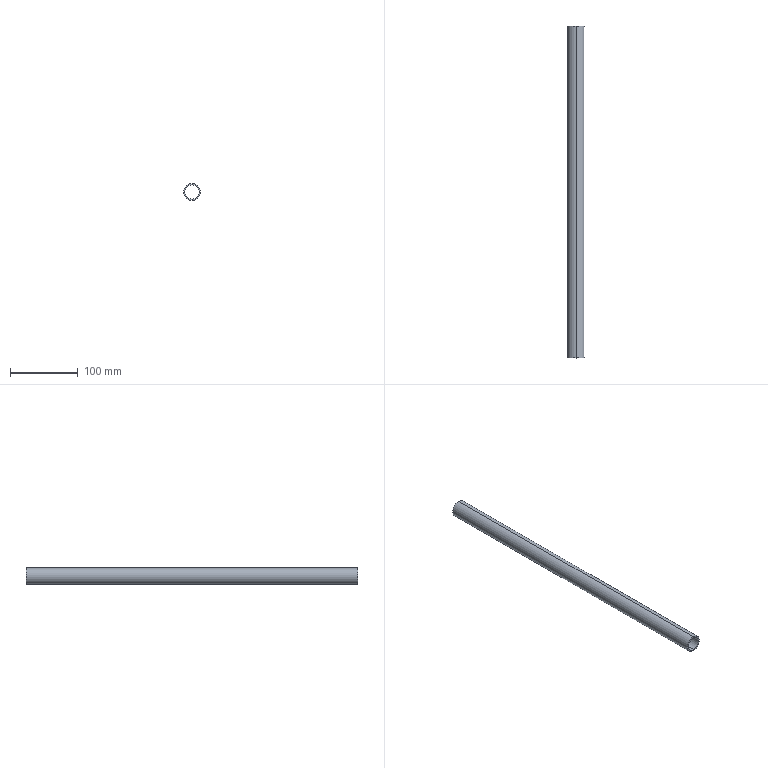Part | STEP file | Central air duct | 1 solid | 6 faces | box 25 x 490 x 25 mm | volume 70811 mm3 | cylinder 4 | plane 2 | commonest cylinder face diameters 21 x2 25 x2
STEP:
#1=CARTESIAN_POINT('',(0.,0.,0.));
#2=DIRECTION('',(0.,0.,1.));
#3=DIRECTION('',(1.,0.,0.));
#4=AXIS2_PLACEMENT_3D('',#1,#2,#3);
#5=CARTESIAN_POINT('',(0.,245.,-10.5));
#6=VERTEX_POINT('',#5);
#7=CARTESIAN_POINT('',(0.,-245.,-10.5));
#8=VERTEX_POINT('',#7);
#9=CARTESIAN_POINT('',(0.,245.,-10.5));
#10=DIRECTION('',(0.,-1.,0.));
#11=VECTOR('',#10,1.);
#12=LINE('',#9,#11);
#13=CARTESIAN_POINT('',(0.,245.,0.));
#14=DIRECTION('',(0.,-1.,0.));
#15=DIRECTION('',(0.,0.,-1.));
#16=AXIS2_PLACEMENT_3D('',#13,#14,#15);
#17=CYLINDRICAL_SURFACE('',#16,10.5);
#18=CARTESIAN_POINT('',(6.283,0.));
#19=DIRECTION('',(0.,1.));
#20=VECTOR('',#19,1.);
#21=LINE('',#18,#20);
#22=(GEOMETRIC_REPRESENTATION_CONTEXT(2)PARAMETRIC_REPRESENTATION_CONTEXT()REPRESENTATION_CONTEXT('',''));
#23=DEFINITIONAL_REPRESENTATION('',(#21),#22);
#24=PCURVE('',#17,#23);
#25=CARTESIAN_POINT('',(0.,245.,0.));
#26=DIRECTION('',(0.,-1.,0.));
#27=DIRECTION('',(0.,0.,-1.));
#28=AXIS2_PLACEMENT_3D('',#25,#26,#27);
#29=CYLINDRICAL_SURFACE('',#28,10.5);
#30=CARTESIAN_POINT('',(0.,0.));
#31=DIRECTION('',(0.,1.));
#32=VECTOR('',#31,1.);
#33=LINE('',#30,#32);
#34=(GEOMETRIC_REPRESENTATION_CONTEXT(2)PARAMETRIC_REPRESENTATION_CONTEXT()REPRESENTATION_CONTEXT('',''));
#35=DEFINITIONAL_REPRESENTATION('',(#33),#34);
#36=PCURVE('',#29,#35);
#37=SURFACE_CURVE('',#12,(#24,#36),.PCURVE_S1.);
#38=EDGE_CURVE('',#6,#8,#37,.T.);
#39=ORIENTED_EDGE('',*,*,#38,.T.);
#40=CARTESIAN_POINT('',(0.,-245.,10.5));
#41=VERTEX_POINT('',#40);
#42=CARTESIAN_POINT('',(0.,-245.,0.));
#43=DIRECTION('',(0.,1.,0.));
#44=DIRECTION('',(1.,0.,0.));
#45=AXIS2_PLACEMENT_3D('',#42,#43,#44);
#46=CIRCLE('',#45,10.5);
#47=CARTESIAN_POINT('',(7.854,490.));
#48=DIRECTION('',(-1.,0.));
#49=VECTOR('',#48,1.);
#50=LINE('',#47,#49);
#51=(GEOMETRIC_REPRESENTATION_CONTEXT(2)PARAMETRIC_REPRESENTATION_CONTEXT()REPRESENTATION_CONTEXT('',''));
#52=DEFINITIONAL_REPRESENTATION('',(#50),#51);
#53=PCURVE('',#17,#52);
#54=CARTESIAN_POINT('',(0.,-245.,0.));
#55=DIRECTION('',(0.,1.,0.));
#56=DIRECTION('',(0.,0.,1.));
#57=AXIS2_PLACEMENT_3D('',#54,#55,#56);
#58=PLANE('',#57);
#59=CARTESIAN_POINT('',(0.,0.));
#60=DIRECTION('',(0.,1.));
#61=AXIS2_PLACEMENT_2D('',#59,#60);
#62=CIRCLE('',#61,10.5);
#63=(GEOMETRIC_REPRESENTATION_CONTEXT(2)PARAMETRIC_REPRESENTATION_CONTEXT()REPRESENTATION_CONTEXT('',''));
#64=DEFINITIONAL_REPRESENTATION('',(#62),#63);
#65=PCURVE('',#58,#64);
#66=SURFACE_CURVE('',#46,(#53,#65),.PCURVE_S1.);
#67=EDGE_CURVE('',#8,#41,#66,.T.);
#68=ORIENTED_EDGE('',*,*,#67,.T.);
#69=CARTESIAN_POINT('',(0.,245.,10.5));
#70=VERTEX_POINT('',#69);
#71=CARTESIAN_POINT('',(0.,245.,10.5));
#72=DIRECTION('',(0.,-1.,0.));
#73=VECTOR('',#72,1.);
#74=LINE('',#71,#73);
#75=CARTESIAN_POINT('',(3.142,0.));
#76=DIRECTION('',(0.,1.));
#77=VECTOR('',#76,1.);
#78=LINE('',#75,#77);
#79=(GEOMETRIC_REPRESENTATION_CONTEXT(2)PARAMETRIC_REPRESENTATION_CONTEXT()REPRESENTATION_CONTEXT('',''));
#80=DEFINITIONAL_REPRESENTATION('',(#78),#79);
#81=PCURVE('',#17,#80);
#82=CARTESIAN_POINT('',(3.142,0.));
#83=DIRECTION('',(0.,1.));
#84=VECTOR('',#83,1.);
#85=LINE('',#82,#84);
#86=(GEOMETRIC_REPRESENTATION_CONTEXT(2)PARAMETRIC_REPRESENTATION_CONTEXT()REPRESENTATION_CONTEXT('',''));
#87=DEFINITIONAL_REPRESENTATION('',(#85),#86);
#88=PCURVE('',#29,#87);
#89=SURFACE_CURVE('',#74,(#81,#88),.PCURVE_S1.);
#90=EDGE_CURVE('',#70,#41,#89,.T.);
#91=ORIENTED_EDGE('',*,*,#90,.F.);
#92=CARTESIAN_POINT('',(0.,245.,0.));
#93=DIRECTION('',(0.,1.,0.));
#94=DIRECTION('',(1.,0.,0.));
#95=AXIS2_PLACEMENT_3D('',#92,#93,#94);
#96=CIRCLE('',#95,10.5);
#97=CARTESIAN_POINT('',(7.854,0.));
#98=DIRECTION('',(-1.,0.));
#99=VECTOR('',#98,1.);
#100=LINE('',#97,#99);
#101=(GEOMETRIC_REPRESENTATION_CONTEXT(2)PARAMETRIC_REPRESENTATION_CONTEXT()REPRESENTATION_CONTEXT('',''));
#102=DEFINITIONAL_REPRESENTATION('',(#100),#101);
#103=PCURVE('',#17,#102);
#104=CARTESIAN_POINT('',(0.,245.,0.));
#105=DIRECTION('',(0.,1.,0.));
#106=DIRECTION('',(0.,0.,1.));
#107=AXIS2_PLACEMENT_3D('',#104,#105,#106);
#108=PLANE('',#107);
#109=CARTESIAN_POINT('',(0.,0.));
#110=DIRECTION('',(0.,1.));
#111=AXIS2_PLACEMENT_2D('',#109,#110);
#112=CIRCLE('',#111,10.5);
#113=(GEOMETRIC_REPRESENTATION_CONTEXT(2)PARAMETRIC_REPRESENTATION_CONTEXT()REPRESENTATION_CONTEXT('',''));
#114=DEFINITIONAL_REPRESENTATION('',(#112),#113);
#115=PCURVE('',#108,#114);
#116=SURFACE_CURVE('',#96,(#103,#115),.PCURVE_S1.);
#117=EDGE_CURVE('',#6,#70,#116,.T.);
#118=ORIENTED_EDGE('',*,*,#117,.F.);
#119=EDGE_LOOP('',(#39,#68,#91,#118));
#120=FACE_BOUND('',#119,.F.);
#121=ADVANCED_FACE('',(#120),#17,.F.);
#122=CARTESIAN_POINT('',(0.,245.,12.5));
#123=VERTEX_POINT('',#122);
#124=CARTESIAN_POINT('',(0.,245.,-12.5));
#125=VERTEX_POINT('',#124);
#126=CARTESIAN_POINT('',(0.,245.,0.));
#127=DIRECTION('',(0.,1.,0.));
#128=DIRECTION('',(0.,0.,1.));
#129=AXIS2_PLACEMENT_3D('',#126,#127,#128);
#130=CIRCLE('',#129,12.5);
#131=CARTESIAN_POINT('',(0.,245.,0.));
#132=DIRECTION('',(0.,-1.,0.));
#133=DIRECTION('',(0.,0.,-1.));
#134=AXIS2_PLACEMENT_3D('',#131,#132,#133);
#135=CYLINDRICAL_SURFACE('',#134,12.5);
#136=CARTESIAN_POINT('',(3.142,0.));
#137=DIRECTION('',(-1.,0.));
#138=VECTOR('',#137,1.);
#139=LINE('',#136,#138);
#140=(GEOMETRIC_REPRESENTATION_CONTEXT(2)PARAMETRIC_REPRESENTATION_CONTEXT()REPRESENTATION_CONTEXT('',''));
#141=DEFINITIONAL_REPRESENTATION('',(#139),#140);
#142=PCURVE('',#135,#141);
#143=CARTESIAN_POINT('',(0.,0.));
#144=DIRECTION('',(1.,0.));
#145=AXIS2_PLACEMENT_2D('',#143,#144);
#146=CIRCLE('',#145,12.5);
#147=(GEOMETRIC_REPRESENTATION_CONTEXT(2)PARAMETRIC_REPRESENTATION_CONTEXT()REPRESENTATION_CONTEXT('',''));
#148=DEFINITIONAL_REPRESENTATION('',(#146),#147);
#149=PCURVE('',#108,#148);
#150=SURFACE_CURVE('',#130,(#142,#149),.PCURVE_S1.);
#151=EDGE_CURVE('',#123,#125,#150,.T.);
#152=ORIENTED_EDGE('',*,*,#151,.F.);
#153=CARTESIAN_POINT('',(0.,-245.,12.5));
#154=VERTEX_POINT('',#153);
#155=CARTESIAN_POINT('',(0.,245.,12.5));
#156=DIRECTION('',(0.,-1.,0.));
#157=VECTOR('',#156,1.);
#158=LINE('',#155,#157);
#159=CARTESIAN_POINT('',(3.142,0.));
#160=DIRECTION('',(0.,1.));
#161=VECTOR('',#160,1.);
#162=LINE('',#159,#161);
#163=(GEOMETRIC_REPRESENTATION_CONTEXT(2)PARAMETRIC_REPRESENTATION_CONTEXT()REPRESENTATION_CONTEXT('',''));
#164=DEFINITIONAL_REPRESENTATION('',(#162),#163);
#165=PCURVE('',#135,#164);
#166=CARTESIAN_POINT('',(0.,245.,0.));
#167=DIRECTION('',(0.,-1.,0.));
#168=DIRECTION('',(0.,0.,-1.));
#169=AXIS2_PLACEMENT_3D('',#166,#167,#168);
#170=CYLINDRICAL_SURFACE('',#169,12.5);
#171=CARTESIAN_POINT('',(3.142,0.));
#172=DIRECTION('',(0.,1.));
#173=VECTOR('',#172,1.);
#174=LINE('',#171,#173);
#175=(GEOMETRIC_REPRESENTATION_CONTEXT(2)PARAMETRIC_REPRESENTATION_CONTEXT()REPRESENTATION_CONTEXT('',''));
#176=DEFINITIONAL_REPRESENTATION('',(#174),#175);
#177=PCURVE('',#170,#176);
#178=SURFACE_CURVE('',#158,(#165,#177),.PCURVE_S1.);
#179=EDGE_CURVE('',#123,#154,#178,.T.);
#180=ORIENTED_EDGE('',*,*,#179,.T.);
#181=CARTESIAN_POINT('',(0.,-245.,-12.5));
#182=VERTEX_POINT('',#181);
#183=CARTESIAN_POINT('',(0.,-245.,0.));
#184=DIRECTION('',(0.,1.,0.));
#185=DIRECTION('',(0.,0.,1.));
#186=AXIS2_PLACEMENT_3D('',#183,#184,#185);
#187=CIRCLE('',#186,12.5);
#188=CARTESIAN_POINT('',(3.142,490.));
#189=DIRECTION('',(-1.,0.));
#190=VECTOR('',#189,1.);
#191=LINE('',#188,#190);
#192=(GEOMETRIC_REPRESENTATION_CONTEXT(2)PARAMETRIC_REPRESENTATION_CONTEXT()REPRESENTATION_CONTEXT('',''));
#193=DEFINITIONAL_REPRESENTATION('',(#191),#192);
#194=PCURVE('',#135,#193);
#195=CARTESIAN_POINT('',(0.,0.));
#196=DIRECTION('',(1.,0.));
#197=AXIS2_PLACEMENT_2D('',#195,#196);
#198=CIRCLE('',#197,12.5);
#199=(GEOMETRIC_REPRESENTATION_CONTEXT(2)PARAMETRIC_REPRESENTATION_CONTEXT()REPRESENTATION_CONTEXT('',''));
#200=DEFINITIONAL_REPRESENTATION('',(#198),#199);
#201=PCURVE('',#58,#200);
#202=SURFACE_CURVE('',#187,(#194,#201),.PCURVE_S1.);
#203=EDGE_CURVE('',#154,#182,#202,.T.);
#204=ORIENTED_EDGE('',*,*,#203,.T.);
#205=CARTESIAN_POINT('',(0.,245.,-12.5));
#206=DIRECTION('',(0.,-1.,0.));
#207=VECTOR('',#206,1.);
#208=LINE('',#205,#207);
#209=CARTESIAN_POINT('',(0.,0.));
#210=DIRECTION('',(0.,1.));
#211=VECTOR('',#210,1.);
#212=LINE('',#209,#211);
#213=(GEOMETRIC_REPRESENTATION_CONTEXT(2)PARAMETRIC_REPRESENTATION_CONTEXT()REPRESENTATION_CONTEXT('',''));
#214=DEFINITIONAL_REPRESENTATION('',(#212),#213);
#215=PCURVE('',#135,#214);
#216=CARTESIAN_POINT('',(6.283,0.));
#217=DIRECTION('',(0.,1.));
#218=VECTOR('',#217,1.);
#219=LINE('',#216,#218);
#220=(GEOMETRIC_REPRESENTATION_CONTEXT(2)PARAMETRIC_REPRESENTATION_CONTEXT()REPRESENTATION_CONTEXT('',''));
#221=DEFINITIONAL_REPRESENTATION('',(#219),#220);
#222=PCURVE('',#170,#221);
#223=SURFACE_CURVE('',#208,(#215,#222),.PCURVE_S1.);
#224=EDGE_CURVE('',#125,#182,#223,.T.);
#225=ORIENTED_EDGE('',*,*,#224,.F.);
#226=EDGE_LOOP('',(#152,#180,#204,#225));
#227=FACE_BOUND('',#226,.T.);
#228=ADVANCED_FACE('',(#227),#135,.T.);
#229=CARTESIAN_POINT('',(0.,245.,0.));
#230=DIRECTION('',(0.,1.,0.));
#231=DIRECTION('',(0.,0.,1.));
#232=AXIS2_PLACEMENT_3D('',#229,#230,#231);
#233=CIRCLE('',#232,12.5);
#234=CARTESIAN_POINT('',(0.,0.));
#235=DIRECTION('',(1.,0.));
#236=AXIS2_PLACEMENT_2D('',#234,#235);
#237=CIRCLE('',#236,12.5);
#238=(GEOMETRIC_REPRESENTATION_CONTEXT(2)PARAMETRIC_REPRESENTATION_CONTEXT()REPRESENTATION_CONTEXT('',''));
#239=DEFINITIONAL_REPRESENTATION('',(#237),#238);
#240=PCURVE('',#108,#239);
#241=CARTESIAN_POINT('',(9.425,0.));
#242=DIRECTION('',(-1.,0.));
#243=VECTOR('',#242,1.);
#244=LINE('',#241,#243);
#245=(GEOMETRIC_REPRESENTATION_CONTEXT(2)PARAMETRIC_REPRESENTATION_CONTEXT()REPRESENTATION_CONTEXT('',''));
#246=DEFINITIONAL_REPRESENTATION('',(#244),#245);
#247=PCURVE('',#170,#246);
#248=SURFACE_CURVE('',#233,(#240,#247),.PCURVE_S1.);
#249=EDGE_CURVE('',#125,#123,#248,.T.);
#250=ORIENTED_EDGE('',*,*,#249,.T.);
#251=ORIENTED_EDGE('',*,*,#151,.T.);
#252=EDGE_LOOP('',(#250,#251));
#253=FACE_BOUND('',#252,.T.);
#254=ORIENTED_EDGE('',*,*,#117,.F.);
#255=CARTESIAN_POINT('',(0.,245.,0.));
#256=DIRECTION('',(0.,1.,0.));
#257=DIRECTION('',(1.,0.,0.));
#258=AXIS2_PLACEMENT_3D('',#255,#256,#257);
#259=CIRCLE('',#258,10.5);
#260=CARTESIAN_POINT('',(0.,0.));
#261=DIRECTION('',(0.,1.));
#262=AXIS2_PLACEMENT_2D('',#260,#261);
#263=CIRCLE('',#262,10.5);
#264=(GEOMETRIC_REPRESENTATION_CONTEXT(2)PARAMETRIC_REPRESENTATION_CONTEXT()REPRESENTATION_CONTEXT('',''));
#265=DEFINITIONAL_REPRESENTATION('',(#263),#264);
#266=PCURVE('',#108,#265);
#267=CARTESIAN_POINT('',(7.854,0.));
#268=DIRECTION('',(-1.,0.));
#269=VECTOR('',#268,1.);
#270=LINE('',#267,#269);
#271=(GEOMETRIC_REPRESENTATION_CONTEXT(2)PARAMETRIC_REPRESENTATION_CONTEXT()REPRESENTATION_CONTEXT('',''));
#272=DEFINITIONAL_REPRESENTATION('',(#270),#271);
#273=PCURVE('',#29,#272);
#274=SURFACE_CURVE('',#259,(#266,#273),.PCURVE_S1.);
#275=EDGE_CURVE('',#70,#6,#274,.T.);
#276=ORIENTED_EDGE('',*,*,#275,.F.);
#277=EDGE_LOOP('',(#254,#276));
#278=FACE_BOUND('',#277,.T.);
#279=ADVANCED_FACE('',(#253,#278),#108,.T.);
#280=CARTESIAN_POINT('',(0.,-245.,0.));
#281=DIRECTION('',(0.,1.,0.));
#282=DIRECTION('',(0.,0.,1.));
#283=AXIS2_PLACEMENT_3D('',#280,#281,#282);
#284=CIRCLE('',#283,12.5);
#285=CARTESIAN_POINT('',(0.,0.));
#286=DIRECTION('',(1.,0.));
#287=AXIS2_PLACEMENT_2D('',#285,#286);
#288=CIRCLE('',#287,12.5);
#289=(GEOMETRIC_REPRESENTATION_CONTEXT(2)PARAMETRIC_REPRESENTATION_CONTEXT()REPRESENTATION_CONTEXT('',''));
#290=DEFINITIONAL_REPRESENTATION('',(#288),#289);
#291=PCURVE('',#58,#290);
#292=CARTESIAN_POINT('',(9.425,490.));
#293=DIRECTION('',(-1.,0.));
#294=VECTOR('',#293,1.);
#295=LINE('',#292,#294);
#296=(GEOMETRIC_REPRESENTATION_CONTEXT(2)PARAMETRIC_REPRESENTATION_CONTEXT()REPRESENTATION_CONTEXT('',''));
#297=DEFINITIONAL_REPRESENTATION('',(#295),#296);
#298=PCURVE('',#170,#297);
#299=SURFACE_CURVE('',#284,(#291,#298),.PCURVE_S1.);
#300=EDGE_CURVE('',#182,#154,#299,.T.);
#301=ORIENTED_EDGE('',*,*,#300,.F.);
#302=ORIENTED_EDGE('',*,*,#203,.F.);
#303=EDGE_LOOP('',(#301,#302));
#304=FACE_BOUND('',#303,.T.);
#305=ORIENTED_EDGE('',*,*,#67,.T.);
#306=CARTESIAN_POINT('',(0.,-245.,0.));
#307=DIRECTION('',(0.,1.,0.));
#308=DIRECTION('',(1.,0.,0.));
#309=AXIS2_PLACEMENT_3D('',#306,#307,#308);
#310=CIRCLE('',#309,10.5);
#311=CARTESIAN_POINT('',(0.,0.));
#312=DIRECTION('',(0.,1.));
#313=AXIS2_PLACEMENT_2D('',#311,#312);
#314=CIRCLE('',#313,10.5);
#315=(GEOMETRIC_REPRESENTATION_CONTEXT(2)PARAMETRIC_REPRESENTATION_CONTEXT()REPRESENTATION_CONTEXT('',''));
#316=DEFINITIONAL_REPRESENTATION('',(#314),#315);
#317=PCURVE('',#58,#316);
#318=CARTESIAN_POINT('',(7.854,490.));
#319=DIRECTION('',(-1.,0.));
#320=VECTOR('',#319,1.);
#321=LINE('',#318,#320);
#322=(GEOMETRIC_REPRESENTATION_CONTEXT(2)PARAMETRIC_REPRESENTATION_CONTEXT()REPRESENTATION_CONTEXT('',''));
#323=DEFINITIONAL_REPRESENTATION('',(#321),#322);
#324=PCURVE('',#29,#323);
#325=SURFACE_CURVE('',#310,(#317,#324),.PCURVE_S1.);
#326=EDGE_CURVE('',#41,#8,#325,.T.);
#327=ORIENTED_EDGE('',*,*,#326,.T.);
#328=EDGE_LOOP('',(#305,#327));
#329=FACE_BOUND('',#328,.T.);
#330=ADVANCED_FACE('',(#304,#329),#58,.F.);
#331=ORIENTED_EDGE('',*,*,#179,.F.);
#332=ORIENTED_EDGE('',*,*,#249,.F.);
#333=ORIENTED_EDGE('',*,*,#224,.T.);
#334=ORIENTED_EDGE('',*,*,#300,.T.);
#335=EDGE_LOOP('',(#331,#332,#333,#334));
#336=FACE_BOUND('',#335,.T.);
#337=ADVANCED_FACE('',(#336),#170,.T.);
#338=ORIENTED_EDGE('',*,*,#326,.T.);
#339=ORIENTED_EDGE('',*,*,#38,.F.);
#340=ORIENTED_EDGE('',*,*,#275,.F.);
#341=ORIENTED_EDGE('',*,*,#90,.T.);
#342=EDGE_LOOP('',(#338,#339,#340,#341));
#343=FACE_BOUND('',#342,.F.);
#344=ADVANCED_FACE('',(#343),#29,.F.);
#345=CLOSED_SHELL('',(#121,#228,#279,#330,#337,#344));
#346=MANIFOLD_SOLID_BREP('',#345);
#347=(LENGTH_UNIT()NAMED_UNIT(*)SI_UNIT(.MILLI.,.METRE.));
#348=UNCERTAINTY_MEASURE_WITH_UNIT(LENGTH_MEASURE(0.0000001),#347,'','');
#349=(NAMED_UNIT(*)PLANE_ANGLE_UNIT()SI_UNIT($,.RADIAN.));
#350=(NAMED_UNIT(*)SI_UNIT($,.STERADIAN.)SOLID_ANGLE_UNIT());
#351=(GEOMETRIC_REPRESENTATION_CONTEXT(3)GLOBAL_UNCERTAINTY_ASSIGNED_CONTEXT((#348))GLOBAL_UNIT_ASSIGNED_CONTEXT((#347,#349,#350))REPRESENTATION_CONTEXT('',''));
#352=ADVANCED_BREP_SHAPE_REPRESENTATION('',(#4,#346),#351);